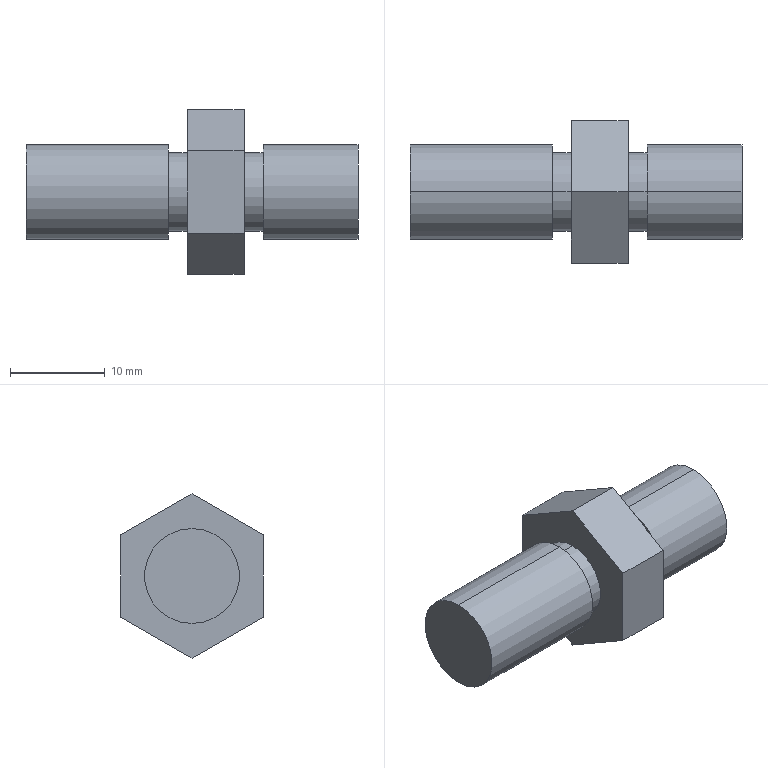Part | SolidWorks | features Revolution 2, Extrusion 1 | 1 solid | 20 faces | box 35 x 15 x 17.321 mm | volume 3350 mm3 | plane 12 | cylinder 8 | commonest cylinder face diameters 8.314 x4 10 x4
STEP:
#1=CARTESIAN_POINT('',(10.,0.,-5.));
#2=VERTEX_POINT('',#1);
#3=CARTESIAN_POINT('',(10.,0.,5.));
#4=VERTEX_POINT('',#3);
#5=CARTESIAN_POINT('',(10.,0.,0.));
#6=DIRECTION('',(1.,0.,0.));
#7=DIRECTION('',(0.,0.,-1.));
#8=AXIS2_PLACEMENT_3D('',#5,#6,#7);
#9=CIRCLE('',#8,5.);
#10=EDGE_CURVE('',#2,#4,#9,.T.);
#11=ORIENTED_EDGE('',*,*,#10,.T.);
#12=CARTESIAN_POINT('',(20.,0.,5.));
#13=VERTEX_POINT('',#12);
#14=CARTESIAN_POINT('',(8.,0.,5.));
#15=DIRECTION('',(1.,0.,0.));
#16=VECTOR('',#15,1000.);
#17=LINE('',#14,#16);
#18=EDGE_CURVE('',#4,#13,#17,.T.);
#19=ORIENTED_EDGE('',*,*,#18,.T.);
#20=CARTESIAN_POINT('',(20.,0.,-5.));
#21=VERTEX_POINT('',#20);
#22=CARTESIAN_POINT('',(20.,0.,0.));
#23=DIRECTION('',(1.,0.,0.));
#24=DIRECTION('',(0.,0.,-1.));
#25=AXIS2_PLACEMENT_3D('',#22,#23,#24);
#26=CIRCLE('',#25,5.);
#27=EDGE_CURVE('',#21,#13,#26,.T.);
#28=ORIENTED_EDGE('',*,*,#27,.F.);
#29=CARTESIAN_POINT('',(8.,0.,-5.));
#30=DIRECTION('',(1.,0.,0.));
#31=VECTOR('',#30,1000.);
#32=LINE('',#29,#31);
#33=EDGE_CURVE('',#2,#21,#32,.T.);
#34=ORIENTED_EDGE('',*,*,#33,.F.);
#35=EDGE_LOOP('',(#11,#19,#28,#34));
#36=FACE_OUTER_BOUND('',#35,.T.);
#37=CARTESIAN_POINT('',(8.,0.,0.));
#38=DIRECTION('',(1.,0.,0.));
#39=DIRECTION('',(0.,0.,-1.));
#40=AXIS2_PLACEMENT_3D('',#37,#38,#39);
#41=CYLINDRICAL_SURFACE('',#40,5.);
#42=ADVANCED_FACE('',(#36),#41,.T.);
#43=CARTESIAN_POINT('',(8.,0.,-4.157));
#44=VERTEX_POINT('',#43);
#45=CARTESIAN_POINT('',(8.,0.,4.157));
#46=VERTEX_POINT('',#45);
#47=CARTESIAN_POINT('',(8.,0.,0.));
#48=DIRECTION('',(1.,0.,0.));
#49=DIRECTION('',(0.,0.,-1.));
#50=AXIS2_PLACEMENT_3D('',#47,#48,#49);
#51=CIRCLE('',#50,4.157);
#52=EDGE_CURVE('',#44,#46,#51,.T.);
#53=ORIENTED_EDGE('',*,*,#52,.T.);
#54=CARTESIAN_POINT('',(10.,0.,4.157));
#55=VERTEX_POINT('',#54);
#56=CARTESIAN_POINT('',(8.,0.,4.157));
#57=DIRECTION('',(1.,0.,0.));
#58=VECTOR('',#57,1000.);
#59=LINE('',#56,#58);
#60=EDGE_CURVE('',#46,#55,#59,.T.);
#61=ORIENTED_EDGE('',*,*,#60,.T.);
#62=CARTESIAN_POINT('',(10.,0.,-4.157));
#63=VERTEX_POINT('',#62);
#64=CARTESIAN_POINT('',(10.,0.,0.));
#65=DIRECTION('',(1.,0.,0.));
#66=DIRECTION('',(0.,0.,-1.));
#67=AXIS2_PLACEMENT_3D('',#64,#65,#66);
#68=CIRCLE('',#67,4.157);
#69=EDGE_CURVE('',#63,#55,#68,.T.);
#70=ORIENTED_EDGE('',*,*,#69,.F.);
#71=CARTESIAN_POINT('',(8.,0.,-4.157));
#72=DIRECTION('',(1.,0.,0.));
#73=VECTOR('',#72,1000.);
#74=LINE('',#71,#73);
#75=EDGE_CURVE('',#44,#63,#74,.T.);
#76=ORIENTED_EDGE('',*,*,#75,.F.);
#77=EDGE_LOOP('',(#53,#61,#70,#76));
#78=FACE_OUTER_BOUND('',#77,.T.);
#79=CARTESIAN_POINT('',(8.,0.,0.));
#80=DIRECTION('',(1.,0.,0.));
#81=DIRECTION('',(0.,0.,-1.));
#82=AXIS2_PLACEMENT_3D('',#79,#80,#81);
#83=CYLINDRICAL_SURFACE('',#82,4.157);
#84=ADVANCED_FACE('',(#78),#83,.T.);
#85=CARTESIAN_POINT('',(0.,0.,-4.157));
#86=VERTEX_POINT('',#85);
#87=CARTESIAN_POINT('',(0.,0.,4.157));
#88=VERTEX_POINT('',#87);
#89=CARTESIAN_POINT('',(0.,0.,0.));
#90=DIRECTION('',(1.,0.,0.));
#91=DIRECTION('',(0.,0.,-1.));
#92=AXIS2_PLACEMENT_3D('',#89,#90,#91);
#93=CIRCLE('',#92,4.157);
#94=EDGE_CURVE('',#86,#88,#93,.T.);
#95=ORIENTED_EDGE('',*,*,#94,.T.);
#96=CARTESIAN_POINT('',(2.,0.,4.157));
#97=VERTEX_POINT('',#96);
#98=CARTESIAN_POINT('',(-15.,0.,4.157));
#99=DIRECTION('',(1.,0.,0.));
#100=VECTOR('',#99,1000.);
#101=LINE('',#98,#100);
#102=EDGE_CURVE('',#88,#97,#101,.T.);
#103=ORIENTED_EDGE('',*,*,#102,.T.);
#104=CARTESIAN_POINT('',(2.,0.,-4.157));
#105=VERTEX_POINT('',#104);
#106=CARTESIAN_POINT('',(2.,0.,0.));
#107=DIRECTION('',(1.,0.,0.));
#108=DIRECTION('',(0.,0.,-1.));
#109=AXIS2_PLACEMENT_3D('',#106,#107,#108);
#110=CIRCLE('',#109,4.157);
#111=EDGE_CURVE('',#105,#97,#110,.T.);
#112=ORIENTED_EDGE('',*,*,#111,.F.);
#113=CARTESIAN_POINT('',(-15.,0.,-4.157));
#114=DIRECTION('',(1.,0.,0.));
#115=VECTOR('',#114,1000.);
#116=LINE('',#113,#115);
#117=EDGE_CURVE('',#86,#105,#116,.T.);
#118=ORIENTED_EDGE('',*,*,#117,.F.);
#119=EDGE_LOOP('',(#95,#103,#112,#118));
#120=FACE_OUTER_BOUND('',#119,.T.);
#121=CARTESIAN_POINT('',(-15.,0.,0.));
#122=DIRECTION('',(1.,0.,0.));
#123=DIRECTION('',(0.,0.,-1.));
#124=AXIS2_PLACEMENT_3D('',#121,#122,#123);
#125=CYLINDRICAL_SURFACE('',#124,4.157);
#126=ADVANCED_FACE('',(#120),#125,.T.);
#127=CARTESIAN_POINT('',(-15.,0.,-5.));
#128=VERTEX_POINT('',#127);
#129=CARTESIAN_POINT('',(-15.,0.,5.));
#130=VERTEX_POINT('',#129);
#131=CARTESIAN_POINT('',(-15.,0.,0.));
#132=DIRECTION('',(1.,0.,0.));
#133=DIRECTION('',(0.,0.,-1.));
#134=AXIS2_PLACEMENT_3D('',#131,#132,#133);
#135=CIRCLE('',#134,5.);
#136=EDGE_CURVE('',#128,#130,#135,.T.);
#137=ORIENTED_EDGE('',*,*,#136,.T.);
#138=CARTESIAN_POINT('',(0.,0.,5.));
#139=VERTEX_POINT('',#138);
#140=CARTESIAN_POINT('',(-15.,0.,5.));
#141=DIRECTION('',(1.,0.,0.));
#142=VECTOR('',#141,1000.);
#143=LINE('',#140,#142);
#144=EDGE_CURVE('',#130,#139,#143,.T.);
#145=ORIENTED_EDGE('',*,*,#144,.T.);
#146=CARTESIAN_POINT('',(0.,0.,-5.));
#147=VERTEX_POINT('',#146);
#148=CARTESIAN_POINT('',(0.,0.,0.));
#149=DIRECTION('',(1.,0.,0.));
#150=DIRECTION('',(0.,0.,-1.));
#151=AXIS2_PLACEMENT_3D('',#148,#149,#150);
#152=CIRCLE('',#151,5.);
#153=EDGE_CURVE('',#147,#139,#152,.T.);
#154=ORIENTED_EDGE('',*,*,#153,.F.);
#155=CARTESIAN_POINT('',(-15.,0.,-5.));
#156=DIRECTION('',(1.,0.,0.));
#157=VECTOR('',#156,1000.);
#158=LINE('',#155,#157);
#159=EDGE_CURVE('',#128,#147,#158,.T.);
#160=ORIENTED_EDGE('',*,*,#159,.F.);
#161=EDGE_LOOP('',(#137,#145,#154,#160));
#162=FACE_OUTER_BOUND('',#161,.T.);
#163=CARTESIAN_POINT('',(-15.,0.,0.));
#164=DIRECTION('',(1.,0.,0.));
#165=DIRECTION('',(0.,0.,-1.));
#166=AXIS2_PLACEMENT_3D('',#163,#164,#165);
#167=CYLINDRICAL_SURFACE('',#166,5.);
#168=ADVANCED_FACE('',(#162),#167,.T.);
#169=CARTESIAN_POINT('',(8.,7.5,4.33));
#170=VERTEX_POINT('',#169);
#171=CARTESIAN_POINT('',(8.,0.,8.66));
#172=VERTEX_POINT('',#171);
#173=CARTESIAN_POINT('',(8.,7.5,4.33));
#174=DIRECTION('',(0.,-0.866,0.5));
#175=VECTOR('',#174,1000.);
#176=LINE('',#173,#175);
#177=EDGE_CURVE('',#170,#172,#176,.T.);
#178=ORIENTED_EDGE('',*,*,#177,.F.);
#179=CARTESIAN_POINT('',(2.,7.5,4.33));
#180=VERTEX_POINT('',#179);
#181=CARTESIAN_POINT('',(2.,7.5,4.33));
#182=DIRECTION('',(1.,0.,0.));
#183=VECTOR('',#182,1000.);
#184=LINE('',#181,#183);
#185=EDGE_CURVE('',#180,#170,#184,.T.);
#186=ORIENTED_EDGE('',*,*,#185,.F.);
#187=CARTESIAN_POINT('',(2.,0.,8.66));
#188=VERTEX_POINT('',#187);
#189=CARTESIAN_POINT('',(2.,7.5,4.33));
#190=DIRECTION('',(0.,-0.866,0.5));
#191=VECTOR('',#190,1000.);
#192=LINE('',#189,#191);
#193=EDGE_CURVE('',#180,#188,#192,.T.);
#194=ORIENTED_EDGE('',*,*,#193,.T.);
#195=CARTESIAN_POINT('',(2.,0.,8.66));
#196=DIRECTION('',(1.,0.,0.));
#197=VECTOR('',#196,1000.);
#198=LINE('',#195,#197);
#199=EDGE_CURVE('',#188,#172,#198,.T.);
#200=ORIENTED_EDGE('',*,*,#199,.T.);
#201=EDGE_LOOP('',(#178,#186,#194,#200));
#202=FACE_OUTER_BOUND('',#201,.T.);
#203=CARTESIAN_POINT('',(2.,7.5,4.33));
#204=DIRECTION('',(0.,0.5,0.866));
#205=DIRECTION('',(0.,-0.866,0.5));
#206=AXIS2_PLACEMENT_3D('',#203,#204,#205);
#207=PLANE('',#206);
#208=ADVANCED_FACE('',(#202),#207,.T.);
#209=CARTESIAN_POINT('',(8.,7.5,-4.33));
#210=VERTEX_POINT('',#209);
#211=CARTESIAN_POINT('',(8.,7.5,-4.33));
#212=DIRECTION('',(0.,0.,1.));
#213=VECTOR('',#212,1000.);
#214=LINE('',#211,#213);
#215=EDGE_CURVE('',#210,#170,#214,.T.);
#216=ORIENTED_EDGE('',*,*,#215,.F.);
#217=CARTESIAN_POINT('',(2.,7.5,-4.33));
#218=VERTEX_POINT('',#217);
#219=CARTESIAN_POINT('',(2.,7.5,-4.33));
#220=DIRECTION('',(1.,0.,0.));
#221=VECTOR('',#220,1000.);
#222=LINE('',#219,#221);
#223=EDGE_CURVE('',#218,#210,#222,.T.);
#224=ORIENTED_EDGE('',*,*,#223,.F.);
#225=CARTESIAN_POINT('',(2.,7.5,-4.33));
#226=DIRECTION('',(0.,0.,1.));
#227=VECTOR('',#226,1000.);
#228=LINE('',#225,#227);
#229=EDGE_CURVE('',#218,#180,#228,.T.);
#230=ORIENTED_EDGE('',*,*,#229,.T.);
#231=ORIENTED_EDGE('',*,*,#185,.T.);
#232=EDGE_LOOP('',(#216,#224,#230,#231));
#233=FACE_OUTER_BOUND('',#232,.T.);
#234=CARTESIAN_POINT('',(2.,7.5,-4.33));
#235=DIRECTION('',(0.,1.,0.));
#236=DIRECTION('',(0.,0.,1.));
#237=AXIS2_PLACEMENT_3D('',#234,#235,#236);
#238=PLANE('',#237);
#239=ADVANCED_FACE('',(#233),#238,.T.);
#240=CARTESIAN_POINT('',(8.,0.,-8.66));
#241=VERTEX_POINT('',#240);
#242=CARTESIAN_POINT('',(8.,0.,-8.66));
#243=DIRECTION('',(0.,0.866,0.5));
#244=VECTOR('',#243,1000.);
#245=LINE('',#242,#244);
#246=EDGE_CURVE('',#241,#210,#245,.T.);
#247=ORIENTED_EDGE('',*,*,#246,.F.);
#248=CARTESIAN_POINT('',(2.,0.,-8.66));
#249=VERTEX_POINT('',#248);
#250=CARTESIAN_POINT('',(2.,0.,-8.66));
#251=DIRECTION('',(1.,0.,0.));
#252=VECTOR('',#251,1000.);
#253=LINE('',#250,#252);
#254=EDGE_CURVE('',#249,#241,#253,.T.);
#255=ORIENTED_EDGE('',*,*,#254,.F.);
#256=CARTESIAN_POINT('',(2.,0.,-8.66));
#257=DIRECTION('',(0.,0.866,0.5));
#258=VECTOR('',#257,1000.);
#259=LINE('',#256,#258);
#260=EDGE_CURVE('',#249,#218,#259,.T.);
#261=ORIENTED_EDGE('',*,*,#260,.T.);
#262=ORIENTED_EDGE('',*,*,#223,.T.);
#263=EDGE_LOOP('',(#247,#255,#261,#262));
#264=FACE_OUTER_BOUND('',#263,.T.);
#265=CARTESIAN_POINT('',(2.,0.,-8.66));
#266=DIRECTION('',(0.,0.5,-0.866));
#267=DIRECTION('',(0.,0.866,0.5));
#268=AXIS2_PLACEMENT_3D('',#265,#266,#267);
#269=PLANE('',#268);
#270=ADVANCED_FACE('',(#264),#269,.T.);
#271=CARTESIAN_POINT('',(8.,-7.5,-4.33));
#272=VERTEX_POINT('',#271);
#273=CARTESIAN_POINT('',(8.,-7.5,-4.33));
#274=DIRECTION('',(0.,0.866,-0.5));
#275=VECTOR('',#274,1000.);
#276=LINE('',#273,#275);
#277=EDGE_CURVE('',#272,#241,#276,.T.);
#278=ORIENTED_EDGE('',*,*,#277,.F.);
#279=CARTESIAN_POINT('',(2.,-7.5,-4.33));
#280=VERTEX_POINT('',#279);
#281=CARTESIAN_POINT('',(2.,-7.5,-4.33));
#282=DIRECTION('',(1.,0.,0.));
#283=VECTOR('',#282,1000.);
#284=LINE('',#281,#283);
#285=EDGE_CURVE('',#280,#272,#284,.T.);
#286=ORIENTED_EDGE('',*,*,#285,.F.);
#287=CARTESIAN_POINT('',(2.,-7.5,-4.33));
#288=DIRECTION('',(0.,0.866,-0.5));
#289=VECTOR('',#288,1000.);
#290=LINE('',#287,#289);
#291=EDGE_CURVE('',#280,#249,#290,.T.);
#292=ORIENTED_EDGE('',*,*,#291,.T.);
#293=ORIENTED_EDGE('',*,*,#254,.T.);
#294=EDGE_LOOP('',(#278,#286,#292,#293));
#295=FACE_OUTER_BOUND('',#294,.T.);
#296=CARTESIAN_POINT('',(2.,-7.5,-4.33));
#297=DIRECTION('',(0.,-0.5,-0.866));
#298=DIRECTION('',(0.,0.866,-0.5));
#299=AXIS2_PLACEMENT_3D('',#296,#297,#298);
#300=PLANE('',#299);
#301=ADVANCED_FACE('',(#295),#300,.T.);
#302=CARTESIAN_POINT('',(8.,-7.5,4.33));
#303=VERTEX_POINT('',#302);
#304=CARTESIAN_POINT('',(8.,-7.5,4.33));
#305=DIRECTION('',(0.,0.,-1.));
#306=VECTOR('',#305,1000.);
#307=LINE('',#304,#306);
#308=EDGE_CURVE('',#303,#272,#307,.T.);
#309=ORIENTED_EDGE('',*,*,#308,.F.);
#310=CARTESIAN_POINT('',(2.,-7.5,4.33));
#311=VERTEX_POINT('',#310);
#312=CARTESIAN_POINT('',(2.,-7.5,4.33));
#313=DIRECTION('',(1.,0.,0.));
#314=VECTOR('',#313,1000.);
#315=LINE('',#312,#314);
#316=EDGE_CURVE('',#311,#303,#315,.T.);
#317=ORIENTED_EDGE('',*,*,#316,.F.);
#318=CARTESIAN_POINT('',(2.,-7.5,4.33));
#319=DIRECTION('',(0.,0.,-1.));
#320=VECTOR('',#319,1000.);
#321=LINE('',#318,#320);
#322=EDGE_CURVE('',#311,#280,#321,.T.);
#323=ORIENTED_EDGE('',*,*,#322,.T.);
#324=ORIENTED_EDGE('',*,*,#285,.T.);
#325=EDGE_LOOP('',(#309,#317,#323,#324));
#326=FACE_OUTER_BOUND('',#325,.T.);
#327=CARTESIAN_POINT('',(2.,-7.5,4.33));
#328=DIRECTION('',(0.,-1.,0.));
#329=DIRECTION('',(0.,0.,-1.));
#330=AXIS2_PLACEMENT_3D('',#327,#328,#329);
#331=PLANE('',#330);
#332=ADVANCED_FACE('',(#326),#331,.T.);
#333=CARTESIAN_POINT('',(8.,0.,8.66));
#334=DIRECTION('',(0.,-0.866,-0.5));
#335=VECTOR('',#334,1000.);
#336=LINE('',#333,#335);
#337=EDGE_CURVE('',#172,#303,#336,.T.);
#338=ORIENTED_EDGE('',*,*,#337,.F.);
#339=ORIENTED_EDGE('',*,*,#199,.F.);
#340=CARTESIAN_POINT('',(2.,0.,8.66));
#341=DIRECTION('',(0.,-0.866,-0.5));
#342=VECTOR('',#341,1000.);
#343=LINE('',#340,#342);
#344=EDGE_CURVE('',#188,#311,#343,.T.);
#345=ORIENTED_EDGE('',*,*,#344,.T.);
#346=ORIENTED_EDGE('',*,*,#316,.T.);
#347=EDGE_LOOP('',(#338,#339,#345,#346));
#348=FACE_OUTER_BOUND('',#347,.T.);
#349=CARTESIAN_POINT('',(2.,0.,8.66));
#350=DIRECTION('',(0.,-0.5,0.866));
#351=DIRECTION('',(0.,-0.866,-0.5));
#352=AXIS2_PLACEMENT_3D('',#349,#350,#351);
#353=PLANE('',#352);
#354=ADVANCED_FACE('',(#348),#353,.T.);
#355=ORIENTED_EDGE('',*,*,#111,.T.);
#356=CARTESIAN_POINT('',(2.,0.,0.));
#357=DIRECTION('',(1.,0.,0.));
#358=DIRECTION('',(0.,0.,-1.));
#359=AXIS2_PLACEMENT_3D('',#356,#357,#358);
#360=CIRCLE('',#359,4.157);
#361=EDGE_CURVE('',#97,#105,#360,.T.);
#362=ORIENTED_EDGE('',*,*,#361,.T.);
#363=EDGE_LOOP('',(#355,#362));
#364=FACE_BOUND('',#363,.T.);
#365=ORIENTED_EDGE('',*,*,#193,.F.);
#366=ORIENTED_EDGE('',*,*,#229,.F.);
#367=ORIENTED_EDGE('',*,*,#260,.F.);
#368=ORIENTED_EDGE('',*,*,#291,.F.);
#369=ORIENTED_EDGE('',*,*,#322,.F.);
#370=ORIENTED_EDGE('',*,*,#344,.F.);
#371=EDGE_LOOP('',(#365,#366,#367,#368,#369,#370));
#372=FACE_OUTER_BOUND('',#371,.T.);
#373=CARTESIAN_POINT('',(2.,0.,0.));
#374=DIRECTION('',(1.,0.,0.));
#375=DIRECTION('',(0.,0.,-1.));
#376=AXIS2_PLACEMENT_3D('',#373,#374,#375);
#377=PLANE('',#376);
#378=ADVANCED_FACE('',(#364,#372),#377,.F.);
#379=ORIENTED_EDGE('',*,*,#52,.F.);
#380=CARTESIAN_POINT('',(8.,0.,0.));
#381=DIRECTION('',(1.,0.,0.));
#382=DIRECTION('',(0.,0.,-1.));
#383=AXIS2_PLACEMENT_3D('',#380,#381,#382);
#384=CIRCLE('',#383,4.157);
#385=EDGE_CURVE('',#46,#44,#384,.T.);
#386=ORIENTED_EDGE('',*,*,#385,.F.);
#387=EDGE_LOOP('',(#379,#386));
#388=FACE_BOUND('',#387,.T.);
#389=ORIENTED_EDGE('',*,*,#177,.T.);
#390=ORIENTED_EDGE('',*,*,#337,.T.);
#391=ORIENTED_EDGE('',*,*,#308,.T.);
#392=ORIENTED_EDGE('',*,*,#277,.T.);
#393=ORIENTED_EDGE('',*,*,#246,.T.);
#394=ORIENTED_EDGE('',*,*,#215,.T.);
#395=EDGE_LOOP('',(#389,#390,#391,#392,#393,#394));
#396=FACE_OUTER_BOUND('',#395,.T.);
#397=CARTESIAN_POINT('',(8.,0.,0.));
#398=DIRECTION('',(1.,0.,0.));
#399=DIRECTION('',(0.,0.,-1.));
#400=AXIS2_PLACEMENT_3D('',#397,#398,#399);
#401=PLANE('',#400);
#402=ADVANCED_FACE('',(#388,#396),#401,.T.);
#403=ORIENTED_EDGE('',*,*,#144,.F.);
#404=CARTESIAN_POINT('',(-15.,0.,0.));
#405=DIRECTION('',(1.,0.,0.));
#406=DIRECTION('',(0.,0.,-1.));
#407=AXIS2_PLACEMENT_3D('',#404,#405,#406);
#408=CIRCLE('',#407,5.);
#409=EDGE_CURVE('',#130,#128,#408,.T.);
#410=ORIENTED_EDGE('',*,*,#409,.T.);
#411=ORIENTED_EDGE('',*,*,#159,.T.);
#412=CARTESIAN_POINT('',(0.,0.,0.));
#413=DIRECTION('',(1.,0.,0.));
#414=DIRECTION('',(0.,0.,-1.));
#415=AXIS2_PLACEMENT_3D('',#412,#413,#414);
#416=CIRCLE('',#415,5.);
#417=EDGE_CURVE('',#139,#147,#416,.T.);
#418=ORIENTED_EDGE('',*,*,#417,.F.);
#419=EDGE_LOOP('',(#403,#410,#411,#418));
#420=FACE_OUTER_BOUND('',#419,.T.);
#421=CARTESIAN_POINT('',(-15.,0.,0.));
#422=DIRECTION('',(1.,0.,0.));
#423=DIRECTION('',(0.,0.,-1.));
#424=AXIS2_PLACEMENT_3D('',#421,#422,#423);
#425=CYLINDRICAL_SURFACE('',#424,5.);
#426=ADVANCED_FACE('',(#420),#425,.T.);
#427=ORIENTED_EDGE('',*,*,#136,.F.);
#428=ORIENTED_EDGE('',*,*,#409,.F.);
#429=EDGE_LOOP('',(#427,#428));
#430=FACE_OUTER_BOUND('',#429,.T.);
#431=CARTESIAN_POINT('',(-15.,5.,0.));
#432=DIRECTION('',(-1.,0.,0.));
#433=DIRECTION('',(0.,0.,1.));
#434=AXIS2_PLACEMENT_3D('',#431,#432,#433);
#435=PLANE('',#434);
#436=ADVANCED_FACE('',(#430),#435,.T.);
#437=ORIENTED_EDGE('',*,*,#102,.F.);
#438=CARTESIAN_POINT('',(0.,0.,0.));
#439=DIRECTION('',(1.,0.,0.));
#440=DIRECTION('',(0.,0.,-1.));
#441=AXIS2_PLACEMENT_3D('',#438,#439,#440);
#442=CIRCLE('',#441,4.157);
#443=EDGE_CURVE('',#88,#86,#442,.T.);
#444=ORIENTED_EDGE('',*,*,#443,.T.);
#445=ORIENTED_EDGE('',*,*,#117,.T.);
#446=ORIENTED_EDGE('',*,*,#361,.F.);
#447=EDGE_LOOP('',(#437,#444,#445,#446));
#448=FACE_OUTER_BOUND('',#447,.T.);
#449=CARTESIAN_POINT('',(-15.,0.,0.));
#450=DIRECTION('',(1.,0.,0.));
#451=DIRECTION('',(0.,0.,-1.));
#452=AXIS2_PLACEMENT_3D('',#449,#450,#451);
#453=CYLINDRICAL_SURFACE('',#452,4.157);
#454=ADVANCED_FACE('',(#448),#453,.T.);
#455=ORIENTED_EDGE('',*,*,#153,.T.);
#456=ORIENTED_EDGE('',*,*,#417,.T.);
#457=EDGE_LOOP('',(#455,#456));
#458=FACE_OUTER_BOUND('',#457,.T.);
#459=ORIENTED_EDGE('',*,*,#94,.F.);
#460=ORIENTED_EDGE('',*,*,#443,.F.);
#461=EDGE_LOOP('',(#459,#460));
#462=FACE_BOUND('',#461,.T.);
#463=CARTESIAN_POINT('',(0.,4.157,0.));
#464=DIRECTION('',(1.,0.,0.));
#465=DIRECTION('',(0.,0.,-1.));
#466=AXIS2_PLACEMENT_3D('',#463,#464,#465);
#467=PLANE('',#466);
#468=ADVANCED_FACE('',(#458,#462),#467,.T.);
#469=ORIENTED_EDGE('',*,*,#60,.F.);
#470=ORIENTED_EDGE('',*,*,#385,.T.);
#471=ORIENTED_EDGE('',*,*,#75,.T.);
#472=CARTESIAN_POINT('',(10.,0.,0.));
#473=DIRECTION('',(1.,0.,0.));
#474=DIRECTION('',(0.,0.,-1.));
#475=AXIS2_PLACEMENT_3D('',#472,#473,#474);
#476=CIRCLE('',#475,4.157);
#477=EDGE_CURVE('',#55,#63,#476,.T.);
#478=ORIENTED_EDGE('',*,*,#477,.F.);
#479=EDGE_LOOP('',(#469,#470,#471,#478));
#480=FACE_OUTER_BOUND('',#479,.T.);
#481=CARTESIAN_POINT('',(8.,0.,0.));
#482=DIRECTION('',(1.,0.,0.));
#483=DIRECTION('',(0.,0.,-1.));
#484=AXIS2_PLACEMENT_3D('',#481,#482,#483);
#485=CYLINDRICAL_SURFACE('',#484,4.157);
#486=ADVANCED_FACE('',(#480),#485,.T.);
#487=ORIENTED_EDGE('',*,*,#27,.T.);
#488=CARTESIAN_POINT('',(20.,0.,0.));
#489=DIRECTION('',(1.,0.,0.));
#490=DIRECTION('',(0.,0.,-1.));
#491=AXIS2_PLACEMENT_3D('',#488,#489,#490);
#492=CIRCLE('',#491,5.);
#493=EDGE_CURVE('',#13,#21,#492,.T.);
#494=ORIENTED_EDGE('',*,*,#493,.T.);
#495=EDGE_LOOP('',(#487,#494));
#496=FACE_OUTER_BOUND('',#495,.T.);
#497=CARTESIAN_POINT('',(20.,0.,0.));
#498=DIRECTION('',(1.,0.,0.));
#499=DIRECTION('',(0.,0.,-1.));
#500=AXIS2_PLACEMENT_3D('',#497,#498,#499);
#501=PLANE('',#500);
#502=ADVANCED_FACE('',(#496),#501,.T.);
#503=ORIENTED_EDGE('',*,*,#18,.F.);
#504=CARTESIAN_POINT('',(10.,0.,0.));
#505=DIRECTION('',(1.,0.,0.));
#506=DIRECTION('',(0.,0.,-1.));
#507=AXIS2_PLACEMENT_3D('',#504,#505,#506);
#508=CIRCLE('',#507,5.);
#509=EDGE_CURVE('',#4,#2,#508,.T.);
#510=ORIENTED_EDGE('',*,*,#509,.T.);
#511=ORIENTED_EDGE('',*,*,#33,.T.);
#512=ORIENTED_EDGE('',*,*,#493,.F.);
#513=EDGE_LOOP('',(#503,#510,#511,#512));
#514=FACE_OUTER_BOUND('',#513,.T.);
#515=CARTESIAN_POINT('',(8.,0.,0.));
#516=DIRECTION('',(1.,0.,0.));
#517=DIRECTION('',(0.,0.,-1.));
#518=AXIS2_PLACEMENT_3D('',#515,#516,#517);
#519=CYLINDRICAL_SURFACE('',#518,5.);
#520=ADVANCED_FACE('',(#514),#519,.T.);
#521=ORIENTED_EDGE('',*,*,#69,.T.);
#522=ORIENTED_EDGE('',*,*,#477,.T.);
#523=EDGE_LOOP('',(#521,#522));
#524=FACE_BOUND('',#523,.T.);
#525=ORIENTED_EDGE('',*,*,#10,.F.);
#526=ORIENTED_EDGE('',*,*,#509,.F.);
#527=EDGE_LOOP('',(#525,#526));
#528=FACE_OUTER_BOUND('',#527,.T.);
#529=CARTESIAN_POINT('',(10.,5.,0.));
#530=DIRECTION('',(-1.,0.,0.));
#531=DIRECTION('',(0.,0.,1.));
#532=AXIS2_PLACEMENT_3D('',#529,#530,#531);
#533=PLANE('',#532);
#534=ADVANCED_FACE('',(#524,#528),#533,.T.);
#535=CLOSED_SHELL('',(#42,#84,#126,#168,#208,#239,#270,#301,#332,#354,#378,#402,#426,#436,#454,#468,#486,#502,#520,#534));
#536=MANIFOLD_SOLID_BREP('',#535);
#537=CARTESIAN_POINT('',(0.,0.,0.));
#538=DIRECTION('',(0.,0.,1.));
#539=DIRECTION('',(1.,0.,0.));
#540=AXIS2_PLACEMENT_3D('',#537,#538,#539);
#541=(LENGTH_UNIT()NAMED_UNIT(*)SI_UNIT(.MILLI.,.METRE.));
#542=UNCERTAINTY_MEASURE_WITH_UNIT(LENGTH_MEASURE(0.00001),#541,'','');
#543=(NAMED_UNIT(*)PLANE_ANGLE_UNIT()SI_UNIT($,.RADIAN.));
#544=(NAMED_UNIT(*)SI_UNIT($,.STERADIAN.)SOLID_ANGLE_UNIT());
#545=(GEOMETRIC_REPRESENTATION_CONTEXT(3)GLOBAL_UNCERTAINTY_ASSIGNED_CONTEXT((#542))GLOBAL_UNIT_ASSIGNED_CONTEXT((#541,#543,#544))REPRESENTATION_CONTEXT('',''));
#546=ADVANCED_BREP_SHAPE_REPRESENTATION('',(#536,#540),#545);